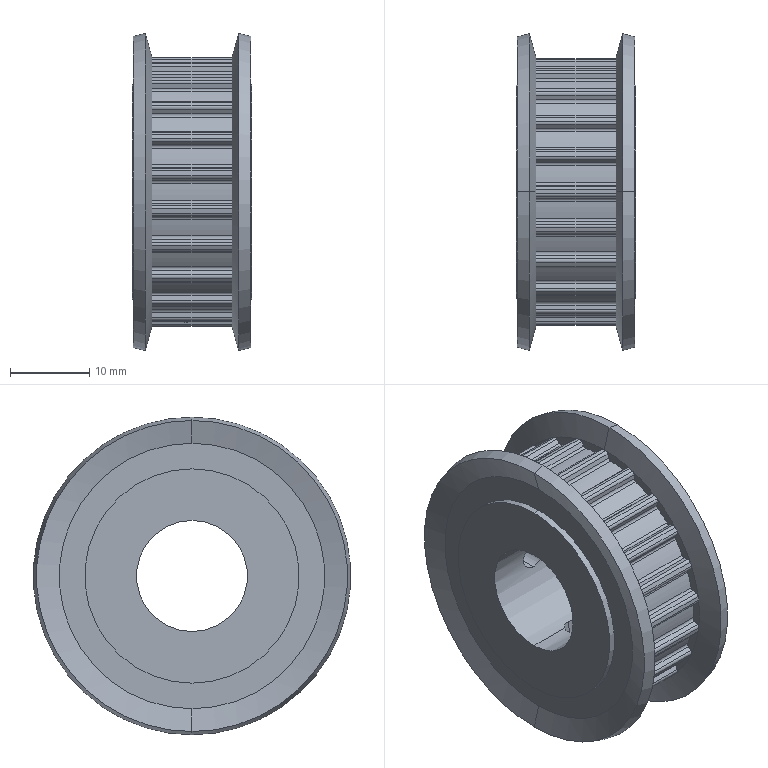Part | STEP file | Synchronous wheel shaft 14V1.201001 | 1 solid | 253 faces | box 15 x 40 x 40 mm | volume 10801 mm3 | cylinder 149 | plane 92 | cone 12 | commonest cylinder face diameters 0.8 x92 31.65 x24 33.85 x23 3.242 x4 27 x4 14 x2